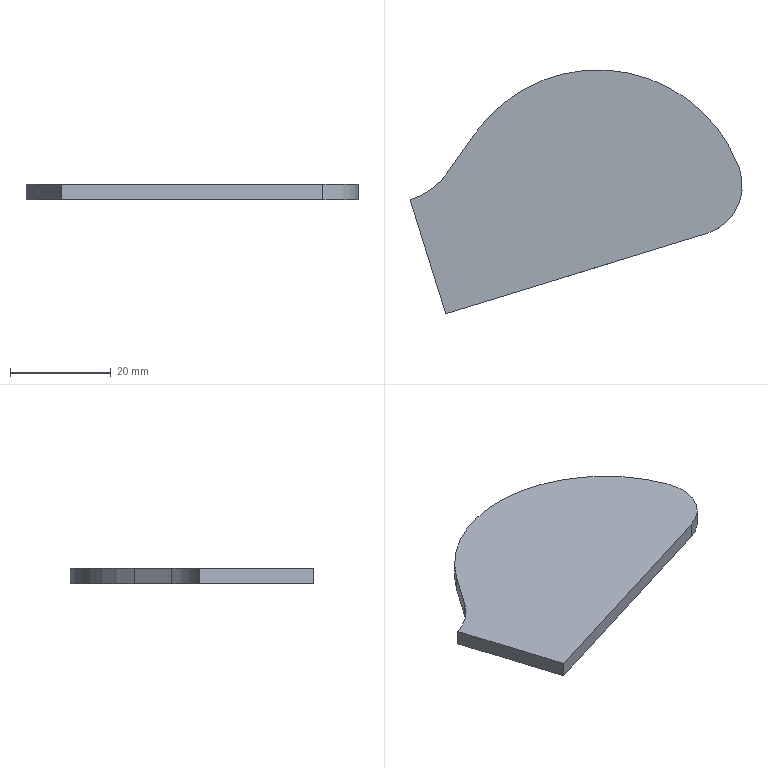Part | SolidWorks | features ICE 4, Fillet 2, BaseBody 1 | 1 solid | 8 faces | box 66.131 x 48.568 x 3 mm | volume 6184 mm3 | plane 5 | cylinder 3 | commonest cylinder face diameters 20 x1 29 x1 60 x1
STEP:
#1=CARTESIAN_POINT('',(11.431,-36.568,3.));
#2=VERTEX_POINT('',#1);
#3=CARTESIAN_POINT('',(4.326,-13.84,3.));
#4=VERTEX_POINT('',#3);
#5=CARTESIAN_POINT('',(19.321,-61.809,3.));
#6=DIRECTION('',(-0.2984,0.9545,0.));
#7=VECTOR('',#6,1000.);
#8=LINE('',#5,#7);
#9=EDGE_CURVE('',#2,#4,#8,.T.);
#10=ORIENTED_EDGE('',*,*,#9,.F.);
#11=CARTESIAN_POINT('',(63.401,-20.562,3.));
#12=VERTEX_POINT('',#11);
#13=CARTESIAN_POINT('',(11.276,-36.615,3.));
#14=DIRECTION('',(-0.9557,-0.2943,0.));
#15=VECTOR('',#14,1000.);
#16=LINE('',#13,#15);
#17=EDGE_CURVE('',#12,#2,#16,.T.);
#18=ORIENTED_EDGE('',*,*,#17,.F.);
#19=CARTESIAN_POINT('',(69.826,-7.508,3.));
#20=VERTEX_POINT('',#19);
#21=CARTESIAN_POINT('',(60.458,-11.005,3.));
#22=DIRECTION('',(0.,0.,1.));
#23=DIRECTION('',(1.,0.,0.));
#24=AXIS2_PLACEMENT_3D('',#21,#22,#23);
#25=CIRCLE('',#24,10.);
#26=EDGE_CURVE('',#12,#20,#25,.T.);
#27=ORIENTED_EDGE('',*,*,#26,.T.);
#28=CARTESIAN_POINT('',(17.146,-0.7927,3.));
#29=VERTEX_POINT('',#28);
#30=CARTESIAN_POINT('',(41.721,-18.,3.));
#31=DIRECTION('',(0.,0.,1.));
#32=DIRECTION('',(-1.,0.,0.));
#33=AXIS2_PLACEMENT_3D('',#30,#31,#32);
#34=CIRCLE('',#33,30.);
#35=EDGE_CURVE('',#20,#29,#34,.T.);
#36=ORIENTED_EDGE('',*,*,#35,.T.);
#37=CARTESIAN_POINT('',(11.878,-8.317,3.));
#38=VERTEX_POINT('',#37);
#39=CARTESIAN_POINT('',(17.146,-0.7927,3.));
#40=DIRECTION('',(-0.5736,-0.8192,0.));
#41=VECTOR('',#40,1000.);
#42=LINE('',#39,#41);
#43=EDGE_CURVE('',#29,#38,#42,.T.);
#44=ORIENTED_EDGE('',*,*,#43,.T.);
#45=CARTESIAN_POINT('',(0.,0.,3.));
#46=DIRECTION('',(0.,0.,-1.));
#47=DIRECTION('',(1.,0.,0.));
#48=AXIS2_PLACEMENT_3D('',#45,#46,#47);
#49=CIRCLE('',#48,14.5);
#50=EDGE_CURVE('',#38,#4,#49,.T.);
#51=ORIENTED_EDGE('',*,*,#50,.T.);
#52=EDGE_LOOP('',(#10,#18,#27,#36,#44,#51));
#53=FACE_OUTER_BOUND('',#52,.T.);
#54=CARTESIAN_POINT('',(-30.124,-77.265,3.));
#55=DIRECTION('',(0.,0.,1.));
#56=DIRECTION('',(1.,0.,0.));
#57=AXIS2_PLACEMENT_3D('',#54,#55,#56);
#58=PLANE('',#57);
#59=ADVANCED_FACE('',(#53),#58,.T.);
#60=CARTESIAN_POINT('',(4.326,-13.84,0.));
#61=VERTEX_POINT('',#60);
#62=CARTESIAN_POINT('',(11.431,-36.568,0.));
#63=VERTEX_POINT('',#62);
#64=CARTESIAN_POINT('',(26.9,-86.052,0.));
#65=DIRECTION('',(0.2984,-0.9545,0.));
#66=VECTOR('',#65,1000.);
#67=LINE('',#64,#66);
#68=EDGE_CURVE('',#61,#63,#67,.T.);
#69=ORIENTED_EDGE('',*,*,#68,.F.);
#70=CARTESIAN_POINT('',(11.878,-8.317,0.));
#71=VERTEX_POINT('',#70);
#72=CARTESIAN_POINT('',(0.,0.,0.));
#73=DIRECTION('',(0.,0.,1.));
#74=DIRECTION('',(1.,0.,0.));
#75=AXIS2_PLACEMENT_3D('',#72,#73,#74);
#76=CIRCLE('',#75,14.5);
#77=EDGE_CURVE('',#61,#71,#76,.T.);
#78=ORIENTED_EDGE('',*,*,#77,.T.);
#79=CARTESIAN_POINT('',(17.146,-0.7927,0.));
#80=VERTEX_POINT('',#79);
#81=CARTESIAN_POINT('',(11.878,-8.317,0.));
#82=DIRECTION('',(0.5736,0.8192,0.));
#83=VECTOR('',#82,1000.);
#84=LINE('',#81,#83);
#85=EDGE_CURVE('',#71,#80,#84,.T.);
#86=ORIENTED_EDGE('',*,*,#85,.T.);
#87=CARTESIAN_POINT('',(69.826,-7.508,0.));
#88=VERTEX_POINT('',#87);
#89=CARTESIAN_POINT('',(41.721,-18.,0.));
#90=DIRECTION('',(0.,0.,-1.));
#91=DIRECTION('',(-1.,0.,0.));
#92=AXIS2_PLACEMENT_3D('',#89,#90,#91);
#93=CIRCLE('',#92,30.);
#94=EDGE_CURVE('',#80,#88,#93,.T.);
#95=ORIENTED_EDGE('',*,*,#94,.T.);
#96=CARTESIAN_POINT('',(63.401,-20.562,0.));
#97=VERTEX_POINT('',#96);
#98=CARTESIAN_POINT('',(60.458,-11.005,0.));
#99=DIRECTION('',(0.,0.,-1.));
#100=DIRECTION('',(-1.,0.,0.));
#101=AXIS2_PLACEMENT_3D('',#98,#99,#100);
#102=CIRCLE('',#101,10.);
#103=EDGE_CURVE('',#88,#97,#102,.T.);
#104=ORIENTED_EDGE('',*,*,#103,.T.);
#105=CARTESIAN_POINT('',(11.276,-36.615,0.));
#106=DIRECTION('',(-0.9557,-0.2943,0.));
#107=VECTOR('',#106,1000.);
#108=LINE('',#105,#107);
#109=EDGE_CURVE('',#97,#63,#108,.T.);
#110=ORIENTED_EDGE('',*,*,#109,.T.);
#111=EDGE_LOOP('',(#69,#78,#86,#95,#104,#110));
#112=FACE_OUTER_BOUND('',#111,.T.);
#113=CARTESIAN_POINT('',(55.01,-77.265,0.));
#114=DIRECTION('',(0.,0.,-1.));
#115=DIRECTION('',(-1.,0.,0.));
#116=AXIS2_PLACEMENT_3D('',#113,#114,#115);
#117=PLANE('',#116);
#118=ADVANCED_FACE('',(#112),#117,.T.);
#119=ORIENTED_EDGE('',*,*,#35,.F.);
#120=CARTESIAN_POINT('',(69.826,-7.508,3.));
#121=DIRECTION('',(0.,0.,-1.));
#122=VECTOR('',#121,1000.);
#123=LINE('',#120,#122);
#124=EDGE_CURVE('',#20,#88,#123,.T.);
#125=ORIENTED_EDGE('',*,*,#124,.T.);
#126=ORIENTED_EDGE('',*,*,#94,.F.);
#127=CARTESIAN_POINT('',(17.146,-0.7927,1.5));
#128=DIRECTION('',(0.,0.,1.));
#129=VECTOR('',#128,1000.);
#130=LINE('',#127,#129);
#131=EDGE_CURVE('',#80,#29,#130,.T.);
#132=ORIENTED_EDGE('',*,*,#131,.T.);
#133=EDGE_LOOP('',(#119,#125,#126,#132));
#134=FACE_OUTER_BOUND('',#133,.T.);
#135=CARTESIAN_POINT('',(41.721,-18.,3.));
#136=DIRECTION('',(0.,0.,-1.));
#137=DIRECTION('',(-1.,0.,0.));
#138=AXIS2_PLACEMENT_3D('',#135,#136,#137);
#139=CYLINDRICAL_SURFACE('',#138,30.);
#140=ADVANCED_FACE('',(#134),#139,.T.);
#141=CARTESIAN_POINT('',(11.878,-8.317,1.5));
#142=DIRECTION('',(0.,0.,1.));
#143=VECTOR('',#142,1000.);
#144=LINE('',#141,#143);
#145=EDGE_CURVE('',#71,#38,#144,.T.);
#146=ORIENTED_EDGE('',*,*,#145,.T.);
#147=ORIENTED_EDGE('',*,*,#43,.F.);
#148=ORIENTED_EDGE('',*,*,#131,.F.);
#149=ORIENTED_EDGE('',*,*,#85,.F.);
#150=EDGE_LOOP('',(#146,#147,#148,#149));
#151=FACE_OUTER_BOUND('',#150,.T.);
#152=CARTESIAN_POINT('',(17.152,-0.7845,-0.01));
#153=DIRECTION('',(-0.8192,0.5736,0.));
#154=DIRECTION('',(-0.5736,-0.8192,0.));
#155=AXIS2_PLACEMENT_3D('',#152,#153,#154);
#156=PLANE('',#155);
#157=ADVANCED_FACE('',(#151),#156,.T.);
#158=CARTESIAN_POINT('',(4.326,-13.84,0.));
#159=DIRECTION('',(0.,0.,-1.));
#160=VECTOR('',#159,1000.);
#161=LINE('',#158,#160);
#162=EDGE_CURVE('',#4,#61,#161,.T.);
#163=ORIENTED_EDGE('',*,*,#162,.F.);
#164=ORIENTED_EDGE('',*,*,#50,.F.);
#165=ORIENTED_EDGE('',*,*,#145,.F.);
#166=ORIENTED_EDGE('',*,*,#77,.F.);
#167=EDGE_LOOP('',(#163,#164,#165,#166));
#168=FACE_OUTER_BOUND('',#167,.T.);
#169=CARTESIAN_POINT('',(0.,0.,0.));
#170=DIRECTION('',(0.,0.,1.));
#171=DIRECTION('',(1.,0.,0.));
#172=AXIS2_PLACEMENT_3D('',#169,#170,#171);
#173=CYLINDRICAL_SURFACE('',#172,14.5);
#174=ADVANCED_FACE('',(#168),#173,.F.);
#175=ORIENTED_EDGE('',*,*,#109,.F.);
#176=CARTESIAN_POINT('',(63.401,-20.562,3.));
#177=DIRECTION('',(0.,0.,1.));
#178=VECTOR('',#177,1000.);
#179=LINE('',#176,#178);
#180=EDGE_CURVE('',#97,#12,#179,.T.);
#181=ORIENTED_EDGE('',*,*,#180,.T.);
#182=ORIENTED_EDGE('',*,*,#17,.T.);
#183=CARTESIAN_POINT('',(11.431,-36.568,0.));
#184=DIRECTION('',(0.,0.,-1.));
#185=VECTOR('',#184,1000.);
#186=LINE('',#183,#185);
#187=EDGE_CURVE('',#2,#63,#186,.T.);
#188=ORIENTED_EDGE('',*,*,#187,.T.);
#189=EDGE_LOOP('',(#175,#181,#182,#188));
#190=FACE_OUTER_BOUND('',#189,.T.);
#191=CARTESIAN_POINT('',(11.276,-36.615,0.));
#192=DIRECTION('',(-0.2943,0.9557,0.));
#193=DIRECTION('',(-0.9557,-0.2943,0.));
#194=AXIS2_PLACEMENT_3D('',#191,#192,#193);
#195=PLANE('',#194);
#196=ADVANCED_FACE('',(#190),#195,.F.);
#197=ORIENTED_EDGE('',*,*,#103,.F.);
#198=ORIENTED_EDGE('',*,*,#124,.F.);
#199=ORIENTED_EDGE('',*,*,#26,.F.);
#200=ORIENTED_EDGE('',*,*,#180,.F.);
#201=EDGE_LOOP('',(#197,#198,#199,#200));
#202=FACE_OUTER_BOUND('',#201,.T.);
#203=CARTESIAN_POINT('',(60.458,-11.005,3.));
#204=DIRECTION('',(0.,0.,-1.));
#205=DIRECTION('',(-1.,0.,0.));
#206=AXIS2_PLACEMENT_3D('',#203,#204,#205);
#207=CYLINDRICAL_SURFACE('',#206,10.);
#208=ADVANCED_FACE('',(#202),#207,.T.);
#209=ORIENTED_EDGE('',*,*,#9,.T.);
#210=ORIENTED_EDGE('',*,*,#162,.T.);
#211=ORIENTED_EDGE('',*,*,#68,.T.);
#212=ORIENTED_EDGE('',*,*,#187,.F.);
#213=EDGE_LOOP('',(#209,#210,#211,#212));
#214=FACE_OUTER_BOUND('',#213,.T.);
#215=CARTESIAN_POINT('',(-15.363,49.146,174.007));
#216=DIRECTION('',(0.9545,0.2984,0.));
#217=DIRECTION('',(-0.2984,0.9545,0.));
#218=AXIS2_PLACEMENT_3D('',#215,#216,#217);
#219=PLANE('',#218);
#220=ADVANCED_FACE('',(#214),#219,.F.);
#221=CLOSED_SHELL('',(#59,#118,#140,#157,#174,#196,#208,#220));
#222=MANIFOLD_SOLID_BREP('',#221);
#223=CARTESIAN_POINT('',(0.,0.,0.));
#224=DIRECTION('',(0.,0.,1.));
#225=DIRECTION('',(1.,0.,0.));
#226=AXIS2_PLACEMENT_3D('',#223,#224,#225);
#227=(LENGTH_UNIT()NAMED_UNIT(*)SI_UNIT(.MILLI.,.METRE.));
#228=UNCERTAINTY_MEASURE_WITH_UNIT(LENGTH_MEASURE(0.00001),#227,'','');
#229=(NAMED_UNIT(*)PLANE_ANGLE_UNIT()SI_UNIT($,.RADIAN.));
#230=(NAMED_UNIT(*)SI_UNIT($,.STERADIAN.)SOLID_ANGLE_UNIT());
#231=(GEOMETRIC_REPRESENTATION_CONTEXT(3)GLOBAL_UNCERTAINTY_ASSIGNED_CONTEXT((#228))GLOBAL_UNIT_ASSIGNED_CONTEXT((#227,#229,#230))REPRESENTATION_CONTEXT('',''));
#232=ADVANCED_BREP_SHAPE_REPRESENTATION('',(#222,#226),#231);